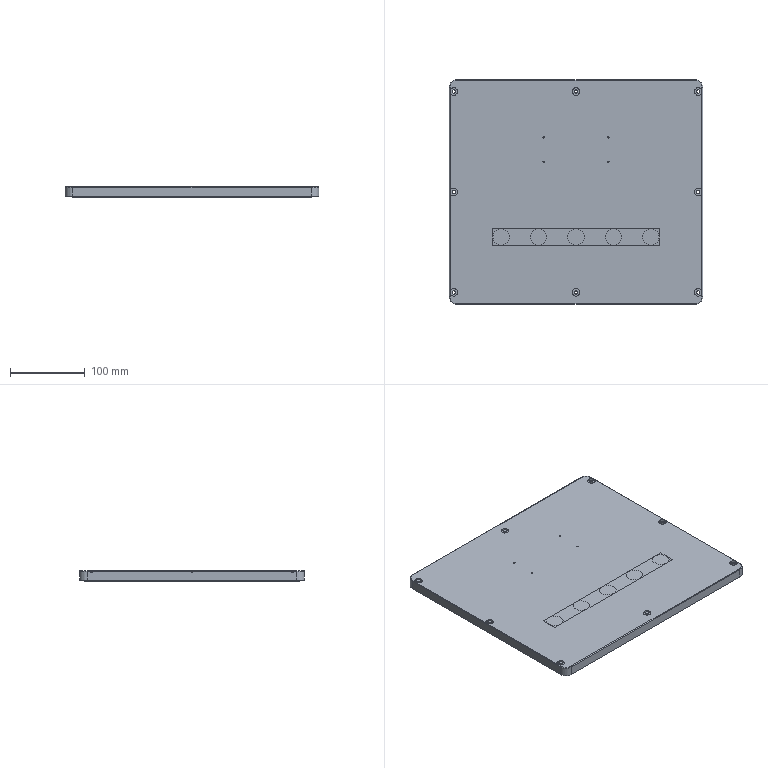NC program | NX | posted with a generic post | part box 338 x 300 x 14.5 mm
Lines 1 to 2601 of 2756, first 2255 of 2575 lines:
N10 G17 G21 G94 G90
(FLOOR_WALL_COPY , TOOL : D63)
N12 T03 M6
N14 G54
N16 G17 G0 G90 X-203.5 Y149.997 S6500 M3
N18 G43 Z30. H3
N20 Z5.662
N22 G94 G1 Z2.662 F1250.
N24 X-200.5
N26 X200.5
N28 Y104.197
N30 X-200.5
N32 Y58.398
N34 X200.5
N36 Y12.599
N38 X-200.5
N40 Y-33.201
N42 X200.5
N44 Y-79.
N46 X-200.5
N48 Y-124.8
N50 X200.5
N52 X203.5
N54 Z5.662
N56 G0 Z30.
N58 X-203.5 Y149.997
N60 Z4.825
N62 G1 Z1.825
N64 X-200.5
N66 X200.5
N68 Y104.197
N70 X-200.5
N72 Y58.398
N74 X200.5
N76 Y12.599
N78 X-200.5
N80 Y-33.201
N82 X200.5
N84 Y-79.
N86 X-200.5
N88 Y-124.8
N90 X200.5
N92 X203.5
N94 Z4.825
N96 G0 Z30.
N98 X-203.5 Y149.997
N100 Z3.987
N102 G1 Z0.987
N104 X-200.5
N106 X200.5
N108 Y104.197
N110 X-200.5
N112 Y58.398
N114 X200.5
N116 Y12.599
N118 X-200.5
N120 Y-33.201
N122 X200.5
N124 Y-79.
N126 X-200.5
N128 Y-124.8
N130 X200.5
N132 X203.5
N134 Z3.987
N136 G0 Z30.
N138 X-203.5 Y149.997
N140 Z3.15
N142 G1 Z0.15
N144 X-200.5
N146 X200.5
N148 Y104.197
N150 X-200.5
N152 Y58.398
N154 X200.5
N156 Y12.599
N158 X-200.5
N160 Y-33.201
N162 X200.5
N164 Y-79.
N166 X-200.5
N168 Y-124.8
N170 X200.5
N172 X203.5
N174 Z3.15
N176 G0 Z30.
(FLOOR_WALL_COPY_1 , TOOL : D63)
N178 X-203.5 Y149.997
N180 Z3.
N182 G1 Z0.
N184 X-200.5
N186 X200.5
N188 Y104.197
N190 X-200.5
N192 Y58.398
N194 X200.5
N196 Y12.599
N198 X-200.5
N200 Y-33.201
N202 X200.5
N204 Y-79.
N206 X-200.5
N208 Y-124.8
N210 X200.5
N212 X203.5
N214 Z3.
N216 G0 Z30.
N218 M5
(CAVITY_MILL_1 , TOOL : D10)
N220 T04 M6
N222 G54
N224 G17 G0 G90 X-3.978 Y-2.05 S9500 M3
N226 G43 Z30. H4
N228 Z1.5
N230 G94 G1 X16.95 Z0.403 F1000.
N232 Y2.05 Z0.188
N234 X0. Z-0.7
N236 X-16.95 F3000.
N238 Y-2.05
N240 X16.95
N242 Y2.05
N244 X0.
N246 Y9.55
N248 X-24.45
N250 Y-9.55
N252 X24.45
N254 Y9.55
N256 X0.
N258 Y17.05
N260 X-31.95
N262 Y-17.05
N264 X31.95
N266 Y17.05
N268 X0.
N270 Y24.55
N272 X-39.45
N274 Y-24.55
N276 X39.45
N278 Y24.55
N280 X0.
N282 Y32.05
N284 X-46.95
N286 Y-32.05
N288 X46.95
N290 Y32.05
N292 X0.
N294 Y39.55
N296 X-54.45
N298 Y-39.55
N300 X54.45
N302 Y39.55
N304 X0.
N306 Y47.05
N308 X-61.95
N310 Y-47.05
N312 X61.95
N314 Y47.05
N316 X0.
N318 Y54.55
N320 X-69.45
N322 Y-54.55
N324 X69.45
N326 Y54.55
N328 X0.
N330 Y62.05
N332 X-76.95
N334 Y-62.05
N336 X76.95
N338 Y62.05
N340 X0.
N342 Y69.55
N344 X-84.45
N346 Y-69.55
N348 X84.45
N350 Y69.55
N352 X0.
N354 Y77.05
N356 X-91.95
N358 Y-77.05
N360 X91.95
N362 Y77.05
N364 X0.
N366 Y84.55
N368 X-99.45
N370 Y-84.55
N372 X99.45
N374 Y84.55
N376 X0.
N378 Y92.05
N380 X-106.95
N382 Y-92.05
N384 X106.95
N386 Y92.05
N388 X0.
N390 Y99.55
N392 X-114.45
N394 Y-99.55
N396 X114.45
N398 Y99.55
N400 X0.
N402 Y107.05
N404 X-121.95
N406 Y-107.05
N408 X121.95
N410 Y107.05
N412 X0.
N414 Y114.55
N416 X-129.45
N418 Y-114.55
N420 X129.45
N422 Y114.55
N424 X0.
N426 Y122.05
N428 X-136.95
N430 Y-122.05
N432 X136.95
N434 Y122.05
N436 X0.
N438 Y129.55
N440 X-144.45
N442 Y-129.55
N444 X144.45
N446 Y129.55
N448 X0.
N450 Y137.05
N452 X-145.05
N454 G3 X-151.95 Y130.15 R6.9
N456 G1 Y-130.15
N458 G3 X-145.05 Y-137.05 R6.9
N460 G1 X145.05
N462 G3 X151.95 Y-130.15 R6.9
N464 G1 Y130.15
N466 G3 X145.05 Y137.05 R6.9
N468 G1 X0.
N470 G3 X-0.866 Y136.55 R1.
N472 G1 Z0.8
N474 G0 Z30.
N476 X-3.978 Y-2.05
N478 Z0.8
N480 G1 X16.95 Z-0.297 F1000.
N482 Y2.05 Z-0.512
N484 X0. Z-1.4
N486 X-16.95 F3000.
N488 Y-2.05
N490 X16.95
N492 Y2.05
N494 X0.
N496 Y9.55
N498 X-24.45
N500 Y-9.55
N502 X24.45
N504 Y9.55
N506 X0.
N508 Y17.05
N510 X-31.95
N512 Y-17.05
N514 X31.95
N516 Y17.05
N518 X0.
N520 Y24.55
N522 X-39.45
N524 Y-24.55
N526 X39.45
N528 Y24.55
N530 X0.
N532 Y32.05
N534 X-46.95
N536 Y-32.05
N538 X46.95
N540 Y32.05
N542 X0.
N544 Y39.55
N546 X-54.45
N548 Y-39.55
N550 X54.45
N552 Y39.55
N554 X0.
N556 Y47.05
N558 X-61.95
N560 Y-47.05
N562 X61.95
N564 Y47.05
N566 X0.
N568 Y54.55
N570 X-69.45
N572 Y-54.55
N574 X69.45
N576 Y54.55
N578 X0.
N580 Y62.05
N582 X-76.95
N584 Y-62.05
N586 X76.95
N588 Y62.05
N590 X0.
N592 Y69.55
N594 X-84.45
N596 Y-69.55
N598 X84.45
N600 Y69.55
N602 X0.
N604 Y77.05
N606 X-91.95
N608 Y-77.05
N610 X91.95
N612 Y77.05
N614 X0.
N616 Y84.55
N618 X-99.45
N620 Y-84.55
N622 X99.45
N624 Y84.55
N626 X0.
N628 Y92.05
N630 X-106.95
N632 Y-92.05
N634 X106.95
N636 Y92.05
N638 X0.
N640 Y99.55
N642 X-114.45
N644 Y-99.55
N646 X114.45
N648 Y99.55
N650 X0.
N652 Y107.05
N654 X-121.95
N656 Y-107.05
N658 X121.95
N660 Y107.05
N662 X0.
N664 Y114.55
N666 X-129.45
N668 Y-114.55
N670 X129.45
N672 Y114.55
N674 X0.
N676 Y122.05
N678 X-136.95
N680 Y-122.05
N682 X136.95
N684 Y122.05
N686 X0.
N688 Y129.55
N690 X-144.45
N692 Y-129.55
N694 X144.45
N696 Y129.55
N698 X0.
N700 Y137.05
N702 X-145.05
N704 G3 X-151.95 Y130.15 R6.9
N706 G1 Y-130.15
N708 G3 X-145.05 Y-137.05 R6.9
N710 G1 X145.05
N712 G3 X151.95 Y-130.15 R6.9
N714 G1 Y130.15
N716 G3 X145.05 Y137.05 R6.9
N718 G1 X0.
N720 G3 X-0.866 Y136.55 R1.
N722 G1 Z0.1
N724 G0 Z30.
N726 X-10.103 Y-1.9
N728 Z0.1
N730 G1 X16.9 Z-1.315 F1000.
N732 Y1.9 Z-1.514
N734 X0. Z-2.4
N736 X-16.9 F3000.
N738 Y-1.9
N740 X16.9
N742 Y1.9
N744 X0.
N746 Y6.4
N748 X-21.4
N750 Y-6.4
N752 X21.4
N754 Y6.4
N756 X0.
N758 Y13.9
N760 X-28.9
N762 Y-13.9
N764 X28.9
N766 Y13.9
N768 X0.
N770 Y21.4
N772 X-36.4
N774 Y-21.4
N776 X36.4
N778 Y21.4
N780 X0.
N782 Y28.9
N784 X-43.9
N786 Y-28.9
N788 X43.9
N790 Y28.9
N792 X0.
N794 Y36.4
N796 X-51.4
N798 Y-36.4
N800 X51.4
N802 Y36.4
N804 X0.
N806 Y43.9
N808 X-58.9
N810 Y-43.9
N812 X58.9
N814 Y43.9
N816 X0.
N818 Y51.4
N820 X-66.4
N822 Y-51.4
N824 X66.4
N826 Y51.4
N828 X0.
N830 Y58.9
N832 X-73.9
N834 Y-58.9
N836 X73.9
N838 Y58.9
N840 X0.
N842 Y66.4
N844 X-81.4
N846 Y-66.4
N848 X81.4
N850 Y66.4
N852 X0.
N854 Y73.9
N856 X-88.9
N858 Y-73.9
N860 X88.9
N862 Y73.9
N864 X0.
N866 Y81.4
N868 X-96.4
N870 Y-81.4
N872 X96.4
N874 Y81.4
N876 X0.
N878 Y88.9
N880 X-103.9
N882 Y-88.9
N884 X103.9
N886 Y88.9
N888 X0.
N890 Y96.4
N892 X-111.4
N894 Y-96.4
N896 X111.4
N898 Y96.4
N900 X0.
N902 Y103.9
N904 X-118.9
N906 Y-103.9
N908 X118.9
N910 Y103.9
N912 X0.
N914 Y111.4
N916 X-126.4
N918 Y-111.4
N920 X126.4
N922 Y111.4
N924 X0.
N926 Y118.9
N928 X-133.9
N930 Y-118.9
N932 X133.9
N934 Y118.9
N936 X0.
N938 Y126.4
N940 X-141.4
N942 Y-126.4
N944 X141.4
N946 Y126.4
N948 X0.
N950 Y133.9
N952 X-144.
N954 G3 X-148.9 Y129. R4.9
N956 G1 Y-129.
N958 G3 X-144. Y-133.9 R4.9
N960 G1 X144.
N962 G3 X148.9 Y-129. R4.9
N964 G1 Y129.
N966 G3 X144. Y133.9 R4.9
N968 G1 X0.
N970 G3 X-0.866 Y133.4 R1.
N972 G1 Z-0.9
N974 G0 X-10.103 Y-1.9
N976 G1 X16.9 Z-2.315 F1000.
N978 Y1.9 Z-2.514
N980 X0. Z-3.4
N982 X-16.9 F3000.
N984 Y-1.9
N986 X16.9
N988 Y1.9
N990 X0.
N992 Y6.4
N994 X-21.4
N996 Y-6.4
N998 X21.4
N1000 Y6.4
N1002 X0.
N1004 Y13.9
N1006 X-28.9
N1008 Y-13.9
N1010 X28.9
N1012 Y13.9
N1014 X0.
N1016 Y21.4
N1018 X-36.4
N1020 Y-21.4
N1022 X36.4
N1024 Y21.4
N1026 X0.
N1028 Y28.9
N1030 X-43.9
N1032 Y-28.9
N1034 X43.9
N1036 Y28.9
N1038 X0.
N1040 Y36.4
N1042 X-51.4
N1044 Y-36.4
N1046 X51.4
N1048 Y36.4
N1050 X0.
N1052 Y43.9
N1054 X-58.9
N1056 Y-43.9
N1058 X58.9
N1060 Y43.9
N1062 X0.
N1064 Y51.4
N1066 X-66.4
N1068 Y-51.4
N1070 X66.4
N1072 Y51.4
N1074 X0.
N1076 Y58.9
N1078 X-73.9
N1080 Y-58.9
N1082 X73.9
N1084 Y58.9
N1086 X0.
N1088 Y66.4
N1090 X-81.4
N1092 Y-66.4
N1094 X81.4
N1096 Y66.4
N1098 X0.
N1100 Y73.9
N1102 X-88.9
N1104 Y-73.9
N1106 X88.9
N1108 Y73.9
N1110 X0.
N1112 Y81.4
N1114 X-96.4
N1116 Y-81.4
N1118 X96.4
N1120 Y81.4
N1122 X0.
N1124 Y88.9
N1126 X-103.9
N1128 Y-88.9
N1130 X103.9
N1132 Y88.9
N1134 X0.
N1136 Y96.4
N1138 X-111.4
N1140 Y-96.4
N1142 X111.4
N1144 Y96.4
N1146 X0.
N1148 Y103.9
N1150 X-118.9
N1152 Y-103.9
N1154 X118.9
N1156 Y103.9
N1158 X0.
N1160 Y111.4
N1162 X-126.4
N1164 Y-111.4
N1166 X126.4
N1168 Y111.4
N1170 X0.
N1172 Y118.9
N1174 X-133.9
N1176 Y-118.9
N1178 X133.9
N1180 Y118.9
N1182 X0.
N1184 Y126.4
N1186 X-141.4
N1188 Y-126.4
N1190 X141.4
N1192 Y126.4
N1194 X0.
N1196 Y133.9
N1198 X-144.
N1200 G3 X-148.9 Y129. R4.9
N1202 G1 Y-129.
N1204 G3 X-144. Y-133.9 R4.9
N1206 G1 X144.
N1208 G3 X148.9 Y-129. R4.9
N1210 G1 Y129.
N1212 G3 X144. Y133.9 R4.9
N1214 G1 X0.
N1216 G3 X-0.866 Y133.4 R1.
N1218 G1 Z-1.9
N1220 G0 X-10.103 Y-1.9
N1222 G1 X16.9 Z-3.315 F1000.
N1224 Y1.9 Z-3.514
N1226 X0. Z-4.4
N1228 X-16.9 F3000.
N1230 Y-1.9
N1232 X16.9
N1234 Y1.9
N1236 X0.
N1238 Y6.4
N1240 X-21.4
N1242 Y-6.4
N1244 X21.4
N1246 Y6.4
N1248 X0.
N1250 Y13.9
N1252 X-28.9
N1254 Y-13.9
N1256 X28.9
N1258 Y13.9
N1260 X0.
N1262 Y21.4
N1264 X-36.4
N1266 Y-21.4
N1268 X36.4
N1270 Y21.4
N1272 X0.
N1274 Y28.9
N1276 X-43.9
N1278 Y-28.9
N1280 X43.9
N1282 Y28.9
N1284 X0.
N1286 Y36.4
N1288 X-51.4
N1290 Y-36.4
N1292 X51.4
N1294 Y36.4
N1296 X0.
N1298 Y43.9
N1300 X-58.9
N1302 Y-43.9
N1304 X58.9
N1306 Y43.9
N1308 X0.
N1310 Y51.4
N1312 X-66.4
N1314 Y-51.4
N1316 X66.4
N1318 Y51.4
N1320 X0.
N1322 Y58.9
N1324 X-73.9
N1326 Y-58.9
N1328 X73.9
N1330 Y58.9
N1332 X0.
N1334 Y66.4
N1336 X-81.4
N1338 Y-66.4
N1340 X81.4
N1342 Y66.4
N1344 X0.
N1346 Y73.9
N1348 X-88.9
N1350 Y-73.9
N1352 X88.9
N1354 Y73.9
N1356 X0.
N1358 Y81.4
N1360 X-96.4
N1362 Y-81.4
N1364 X96.4
N1366 Y81.4
N1368 X0.
N1370 Y88.9
N1372 X-103.9
N1374 Y-88.9
N1376 X103.9
N1378 Y88.9
N1380 X0.
N1382 Y96.4
N1384 X-111.4
N1386 Y-96.4
N1388 X111.4
N1390 Y96.4
N1392 X0.
N1394 Y103.9
N1396 X-118.9
N1398 Y-103.9
N1400 X118.9
N1402 Y103.9
N1404 X0.
N1406 Y111.4
N1408 X-126.4
N1410 Y-111.4
N1412 X126.4
N1414 Y111.4
N1416 X0.
N1418 Y118.9
N1420 X-133.9
N1422 Y-118.9
N1424 X133.9
N1426 Y118.9
N1428 X0.
N1430 Y126.4
N1432 X-141.4
N1434 Y-126.4
N1436 X141.4
N1438 Y126.4
N1440 X0.
N1442 Y133.9
N1444 X-144.
N1446 G3 X-148.9 Y129. R4.9
N1448 G1 Y-129.
N1450 G3 X-144. Y-133.9 R4.9
N1452 G1 X144.
N1454 G3 X148.9 Y-129. R4.9
N1456 G1 Y129.
N1458 G3 X144. Y133.9 R4.9
N1460 G1 X0.
N1462 G3 X-0.866 Y133.4 R1.
N1464 G1 Z-2.9
N1466 G0 X-10.103 Y-1.9
N1468 G1 X16.9 Z-4.315 F1000.
N1470 Y1.9 Z-4.514
N1472 X0. Z-5.4
N1474 X-16.9 F3000.
N1476 Y-1.9
N1478 X16.9
N1480 Y1.9
N1482 X0.
N1484 Y6.4
N1486 X-21.4
N1488 Y-6.4
N1490 X21.4
N1492 Y6.4
N1494 X0.
N1496 Y13.9
N1498 X-28.9
N1500 Y-13.9
N1502 X28.9
N1504 Y13.9
N1506 X0.
N1508 Y21.4
N1510 X-36.4
N1512 Y-21.4
N1514 X36.4
N1516 Y21.4
N1518 X0.
N1520 Y28.9
N1522 X-43.9
N1524 Y-28.9
N1526 X43.9
N1528 Y28.9
N1530 X0.
N1532 Y36.4
N1534 X-51.4
N1536 Y-36.4
N1538 X51.4
N1540 Y36.4
N1542 X0.
N1544 Y43.9
N1546 X-58.9
N1548 Y-43.9
N1550 X58.9
N1552 Y43.9
N1554 X0.
N1556 Y51.4
N1558 X-66.4
N1560 Y-51.4
N1562 X66.4
N1564 Y51.4
N1566 X0.
N1568 Y58.9
N1570 X-73.9
N1572 Y-58.9
N1574 X73.9
N1576 Y58.9
N1578 X0.
N1580 Y66.4
N1582 X-81.4
N1584 Y-66.4
N1586 X81.4
N1588 Y66.4
N1590 X0.
N1592 Y73.9
N1594 X-88.9
N1596 Y-73.9
N1598 X88.9
N1600 Y73.9
N1602 X0.
N1604 Y81.4
N1606 X-96.4
N1608 Y-81.4
N1610 X96.4
N1612 Y81.4
N1614 X0.
N1616 Y88.9
N1618 X-103.9
N1620 Y-88.9
N1622 X103.9
N1624 Y88.9
N1626 X0.
N1628 Y96.4
N1630 X-111.4
N1632 Y-96.4
N1634 X111.4
N1636 Y96.4
N1638 X0.
N1640 Y103.9
N1642 X-118.9
N1644 Y-103.9
N1646 X118.9
N1648 Y103.9
N1650 X0.
N1652 Y111.4
N1654 X-126.4
N1656 Y-111.4
N1658 X126.4
N1660 Y111.4
N1662 X0.
N1664 Y118.9
N1666 X-133.9
N1668 Y-118.9
N1670 X133.9
N1672 Y118.9
N1674 X0.
N1676 Y126.4
N1678 X-141.4
N1680 Y-126.4
N1682 X141.4
N1684 Y126.4
N1686 X0.
N1688 Y133.9
N1690 X-144.
N1692 G3 X-148.9 Y129. R4.9
N1694 G1 Y-129.
N1696 G3 X-144. Y-133.9 R4.9
N1698 G1 X144.
N1700 G3 X148.9 Y-129. R4.9
N1702 G1 Y129.
N1704 G3 X144. Y133.9 R4.9
N1706 G1 X0.
N1708 G3 X-0.866 Y133.4 R1.
N1710 G1 Z-3.9
N1712 G0 X17.397 Y6.6
N1714 G1 X28.9 Z-4.503 F1000.
N1716 Y13.9 Z-4.885
N1718 X0. Z-6.4
N1720 X-28.9 F3000.
N1722 Y6.6
N1724 X28.9
N1726 Y13.9
N1728 X0.
N1730 Y21.4
N1732 X-36.4
N1734 Y-0.9
N1736 X36.4
N1738 Y21.4
N1740 X0.
N1742 Y28.9
N1744 X-43.9
N1746 Y-8.4
N1748 X43.9
N1750 Y28.9
N1752 X0.
N1754 Y36.4
N1756 X-51.4
N1758 Y-15.9
N1760 X51.4
N1762 Y36.4
N1764 X0.
N1766 Y43.9
N1768 X-58.9
N1770 Y-23.4
N1772 X58.9
N1774 Y43.9
N1776 X0.
N1778 Y51.4
N1780 X-66.4
N1782 Y-30.9
N1784 X66.4
N1786 Y51.4
N1788 X0.
N1790 Y58.9
N1792 X-73.9
N1794 Y-38.4
N1796 X73.9
N1798 Y58.9
N1800 X0.
N1802 Y66.4
N1804 X-81.4
N1806 Y-45.9
N1808 X81.4
N1810 Y66.4
N1812 X0.
N1814 Y73.9
N1816 X-88.9
N1818 Y-53.4
N1820 X88.9
N1822 Y73.9
N1824 X0.
N1826 Y81.4
N1828 X-96.4
N1830 Y-60.9
N1832 X96.4
N1834 Y81.4
N1836 X0.
N1838 Y88.9
N1840 X-103.9
N1842 Y-68.4
N1844 X103.9
N1846 Y88.9
N1848 X0.
N1850 Y96.4
N1852 X-111.4
N1854 Y-77.004
N1856 G2 X-105. Y-75.9 R19.1
N1858 G1 X105.
N1860 G2 X111.4 Y-77.004 R19.1
N1862 G1 Y96.4
N1864 X0.
N1866 Y103.9
N1868 X-118.9
N1870 Y-103.9
N1872 X-112.44
N1874 X-107.761 Y-106.337
N1876 X-112.44 Y-103.9
N1878 G2 X-105. Y-83.4 R11.6
N1880 G1 X105.
N1882 G2 X112.44 Y-103.9 R11.6
N1884 G1 X107.761 Y-106.337
N1886 X112.44 Y-103.9
N1888 X111.478 Y-102.749
N1890 G2 X105. Y-105.1 R10.1
N1892 G1 X-105.
N1894 G2 X-115.1 Y-95. R10.1
N1896 X-105. Y-84.9 R10.1
N1898 G1 X105.
N1900 G2 X111.478 Y-102.749 R10.1
N1902 G1 X112.44 Y-103.9
N1904 X118.9
N1906 Y103.9
N1908 X0.
N1910 Y111.4
N1912 X-126.4
N1914 Y-111.4
N1916 X126.4
N1918 Y111.4
N1920 X0.
N1922 Y118.9
N1924 X-133.9
N1926 Y-118.9
N1928 X133.9
N1930 Y118.9
N1932 X0.
N1934 Y126.4
N1936 X-141.4
N1938 Y-126.4
N1940 X141.4
N1942 Y126.4
N1944 X0.
N1946 Y133.9
N1948 X-144.
N1950 G3 X-148.9 Y129. R4.9
N1952 G1 Y-129.
N1954 G3 X-144. Y-133.9 R4.9
N1956 G1 X144.
N1958 G3 X148.9 Y-129. R4.9
N1960 G1 Y129.
N1962 G3 X144. Y133.9 R4.9
N1964 G1 X0.
N1966 G3 X-0.866 Y133.4 R1.
N1968 G1 Z-4.9
N1970 G0 X17.397 Y6.6
N1972 G1 X28.9 Z-5.503 F1000.
N1974 Y13.9 Z-5.885
N1976 X0. Z-7.4
N1978 X-28.9 F3000.
N1980 Y6.6
N1982 X28.9
N1984 Y13.9
N1986 X0.
N1988 Y21.4
N1990 X-36.4
N1992 Y-0.9
N1994 X36.4
N1996 Y21.4
N1998 X0.
N2000 Y28.9
N2002 X-43.9
N2004 Y-8.4
N2006 X43.9
N2008 Y28.9
N2010 X0.
N2012 Y36.4
N2014 X-51.4
N2016 Y-15.9
N2018 X51.4
N2020 Y36.4
N2022 X0.
N2024 Y43.9
N2026 X-58.9
N2028 Y-23.4
N2030 X58.9
N2032 Y43.9
N2034 X0.
N2036 Y51.4
N2038 X-66.4
N2040 Y-30.9
N2042 X66.4
N2044 Y51.4
N2046 X0.
N2048 Y58.9
N2050 X-73.9
N2052 Y-38.4
N2054 X73.9
N2056 Y58.9
N2058 X0.
N2060 Y66.4
N2062 X-81.4
N2064 Y-45.9
N2066 X81.4
N2068 Y66.4
N2070 X0.
N2072 Y73.9
N2074 X-88.9
N2076 Y-53.4
N2078 X88.9
N2080 Y73.9
N2082 X0.
N2084 Y81.4
N2086 X-96.4
N2088 Y-60.9
N2090 X96.4
N2092 Y81.4
N2094 X0.
N2096 Y88.9
N2098 X-103.9
N2100 Y-68.4
N2102 X103.9
N2104 Y88.9
N2106 X0.
N2108 Y96.4
N2110 X-111.4
N2112 Y-77.004
N2114 G2 X-105. Y-75.9 R19.1
N2116 G1 X105.
N2118 G2 X111.4 Y-77.004 R19.1
N2120 G1 Y96.4
N2122 X0.
N2124 Y103.9
N2126 X-118.9
N2128 Y-103.9
N2130 X-112.44
N2132 X-107.761 Y-106.337
N2134 X-112.44 Y-103.9
N2136 G2 X-105. Y-83.4 R11.6
N2138 G1 X105.
N2140 G2 X112.44 Y-103.9 R11.6
N2142 G1 X107.761 Y-106.337
N2144 X112.44 Y-103.9
N2146 X111.478 Y-102.749
N2148 G2 X105. Y-105.1 R10.1
N2150 G1 X-105.
N2152 G2 X-115.1 Y-95. R10.1
N2154 X-105. Y-84.9 R10.1
N2156 G1 X105.
N2158 G2 X111.478 Y-102.749 R10.1
N2160 G1 X112.44 Y-103.9
N2162 X118.9
N2164 Y103.9
N2166 X0.
N2168 Y111.4
N2170 X-126.4
N2172 Y-111.4
N2174 X126.4
N2176 Y111.4
N2178 X0.
N2180 Y118.9
N2182 X-133.9
N2184 Y-118.9
N2186 X133.9
N2188 Y118.9
N2190 X0.
N2192 Y126.4
N2194 X-141.4
N2196 Y-126.4
N2198 X141.4
N2200 Y126.4
N2202 X0.
N2204 Y133.9
N2206 X-144.
N2208 G3 X-148.9 Y129. R4.9
N2210 G1 Y-129.
N2212 G3 X-144. Y-133.9 R4.9
N2214 G1 X144.
N2216 G3 X148.9 Y-129. R4.9
N2218 G1 Y129.
N2220 G3 X144. Y133.9 R4.9
N2222 G1 X0.
N2224 G3 X-0.866 Y133.4 R1.
N2226 G1 Z-5.9
N2228 G0 X17.397 Y6.6
N2230 G1 X28.9 Z-6.503 F1000.
N2232 Y13.9 Z-6.885
N2234 X0. Z-8.4
N2236 X-28.9 F3000.
N2238 Y6.6
N2240 X28.9
N2242 Y13.9
N2244 X0.
N2246 Y21.4
N2248 X-36.4
N2250 Y-0.9
N2252 X36.4
N2254 Y21.4
N2256 X0.
N2258 Y28.9
N2260 X-43.9
N2262 Y-8.4
N2264 X43.9
N2266 Y28.9
N2268 X0.
N2270 Y36.4
N2272 X-51.4
N2274 Y-15.9
N2276 X51.4
N2278 Y36.4
N2280 X0.
N2282 Y43.9
N2284 X-58.9
N2286 Y-23.4
N2288 X58.9
N2290 Y43.9
N2292 X0.
N2294 Y51.4
N2296 X-66.4
N2298 Y-30.9
N2300 X66.4
N2302 Y51.4
N2304 X0.
N2306 Y58.9
N2308 X-73.9
N2310 Y-38.4
N2312 X73.9
N2314 Y58.9
N2316 X0.
N2318 Y66.4
N2320 X-81.4
N2322 Y-45.9
N2324 X81.4
N2326 Y66.4
N2328 X0.
N2330 Y73.9
N2332 X-88.9
N2334 Y-53.4
N2336 X88.9
N2338 Y73.9
N2340 X0.
N2342 Y81.4
N2344 X-96.4
N2346 Y-60.9
N2348 X96.4
N2350 Y81.4
N2352 X0.
N2354 Y88.9
N2356 X-103.9
N2358 Y-68.4
N2360 X103.9
N2362 Y88.9
N2364 X0.
N2366 Y96.4
N2368 X-111.4
N2370 Y-77.004
N2372 G2 X-105. Y-75.9 R19.1
N2374 G1 X105.
N2376 G2 X111.4 Y-77.004 R19.1
N2378 G1 Y96.4
N2380 X0.
N2382 Y103.9
N2384 X-118.9
N2386 Y-103.9
N2388 X-112.44
N2390 X-107.761 Y-106.337
N2392 X-112.44 Y-103.9
N2394 G2 X-105. Y-83.4 R11.6
N2396 G1 X105.
N2398 G2 X112.44 Y-103.9 R11.6
N2400 G1 X107.761 Y-106.337
N2402 X112.44 Y-103.9
N2404 X111.478 Y-102.749
N2406 G2 X105. Y-105.1 R10.1
N2408 G1 X-105.
N2410 G2 X-115.1 Y-95. R10.1
N2412 X-105. Y-84.9 R10.1
N2414 G1 X105.
N2416 G2 X111.478 Y-102.749 R10.1
N2418 G1 X112.44 Y-103.9
N2420 X118.9
N2422 Y103.9
N2424 X0.
N2426 Y111.4
N2428 X-126.4
N2430 Y-111.4
N2432 X126.4
N2434 Y111.4
N2436 X0.
N2438 Y118.9
N2440 X-133.9
N2442 Y-118.9
N2444 X133.9
N2446 Y118.9
N2448 X0.
N2450 Y126.4
N2452 X-141.4
N2454 Y-126.4
N2456 X141.4
N2458 Y126.4
N2460 X0.
N2462 Y133.9
N2464 X-144.
N2466 G3 X-148.9 Y129. R4.9
N2468 G1 Y-129.
N2470 G3 X-144. Y-133.9 R4.9
N2472 G1 X144.
N2474 G3 X148.9 Y-129. R4.9
N2476 G1 Y129.
N2478 G3 X144. Y133.9 R4.9
N2480 G1 X0.
N2482 G3 X-0.866 Y133.4 R1.
N2484 G1 Z-6.9
N2486 G0 X17.397 Y6.6
N2488 G1 X28.9 Z-7.503 F1000.
N2490 Y13.9 Z-7.885
N2492 X0. Z-9.4
N2494 X-28.9 F3000.
N2496 Y6.6
N2498 X28.9
N2500 Y13.9
N2502 X0.
N2504 Y21.4
N2506 X-36.4
N2508 Y-0.9
N2510 X36.4
N2512 Y21.4
N2514 X0.
N2516 Y28.9
N2518 X-43.9
N2520 Y-8.4
N2522 X43.9
N2524 Y28.9
N2526 X0.
N2528 Y36.4
N2530 X-51.4
N2532 Y-15.9
N2534 X51.4
N2536 Y36.4
N2538 X0.
N2540 Y43.9
N2542 X-58.9
N2544 Y-23.4
N2546 X58.9
N2548 Y43.9
N2550 X0.
N2552 Y51.4
N2554 X-66.4
N2556 Y-30.9
N2558 X66.4
N2560 Y51.4
N2562 X0.
N2564 Y58.9
N2566 X-73.9
N2568 Y-38.4
N2570 X73.9
N2572 Y58.9
N2574 X0.
N2576 Y66.4
N2578 X-81.4
N2580 Y-45.9
N2582 X81.4
N2584 Y66.4
N2586 X0.
N2588 Y73.9
N2590 X-88.9
N2592 Y-53.4
N2594 X88.9
N2596 Y73.9
N2598 X0.
N2600 Y81.4
N2602 X-96.4
N2604 Y-60.9
N2606 X96.4
N2608 Y81.4
N2610 X0.
N2612 Y88.9
N2614 X-103.9
N2616 Y-68.4
N2618 X103.9
N2620 Y88.9
N2622 X0.
N2624 Y96.4
N2626 X-111.4
N2628 Y-77.004
N2630 G2 X-105. Y-75.9 R19.1
N2632 G1 X105.
N2634 G2 X111.4 Y-77.004 R19.1
N2636 G1 Y96.4
N2638 X0.
N2640 Y103.9
N2642 X-118.9
N2644 Y-103.9
N2646 X-112.44
N2648 X-107.761 Y-106.337
N2650 X-112.44 Y-103.9
N2652 G2 X-105. Y-83.4 R11.6
N2654 G1 X105.
N2656 G2 X112.44 Y-103.9 R11.6
N2658 G1 X107.761 Y-106.337
N2660 X112.44 Y-103.9
N2662 X111.478 Y-102.749
N2664 G2 X105. Y-105.1 R10.1
N2666 G1 X-105.
N2668 G2 X-115.1 Y-95. R10.1
N2670 X-105. Y-84.9 R10.1
N2672 G1 X105.
N2674 G2 X111.478 Y-102.749 R10.1
N2676 G1 X112.44 Y-103.9
N2678 X118.9
N2680 Y103.9
N2682 X0.
N2684 Y111.4
N2686 X-126.4
N2688 Y-111.4
N2690 X126.4
N2692 Y111.4
N2694 X0.
N2696 Y118.9
N2698 X-133.9
N2700 Y-118.9
N2702 X133.9
N2704 Y118.9
N2706 X0.
N2708 Y126.4
N2710 X-141.4
N2712 Y-126.4
N2714 X141.4
N2716 Y126.4
N2718 X0.
N2720 Y133.9
N2722 X-144.
N2724 G3 X-148.9 Y129. R4.9
N2726 G1 Y-129.
N2728 G3 X-144. Y-133.9 R4.9
N2730 G1 X144.
N2732 G3 X148.9 Y-129. R4.9
N2734 G1 Y129.
N2736 G3 X144. Y133.9 R4.9
N2738 G1 X0.
N2740 G3 X-0.866 Y133.4 R1.
N2742 G1 Z-7.9
N2744 G0 Z30.
(FLOOR_WALL_1 , TOOL : D10)
N2746 X177. Y5.196
N2748 Z0.8
N2750 G1 Z-0.7 F1000.
N2752 X169.5 Y0.866
N2754 G3 X169. Y0. R1.
N2756 G1 Y-140. F2500.
N2758 G2 X159. Y-150. R10.
N2760 G1 X148.794
N2762 G3 X165.25 Y-130.15 R20.2
N2764 G1 Y130.15
N2766 G3 X148.794 Y150. R20.2
N2768 G1 X159.
N2770 G2 X169. Y140. R10.
N2772 G1 Y0.
N2774 G3 X169.5 Y-0.866 R1.
N2776 G1 X177. Y-5.196
N2778 Z0.8
N2780 G0 Z30.
N2782 X-177.
N2784 Z0.8
N2786 G1 Z-0.7 F1000.
N2788 X-169.5 Y-0.866
N2790 G3 X-169. Y0. R1.
N2792 G1 Y140. F2500.
N2794 G2 X-159. Y150. R10.
N2796 G1 X-148.794
N2798 G3 X-165.25 Y130.15 R20.2
N2800 G1 Y-130.15
N2802 G3 X-148.794 Y-150. R20.2
N2804 G1 X-148.535 Y-148.624
N2806 G2 X-163.85 Y-130.15 R18.8
N2808 G1 Y130.15
N2810 G2 X-145.05 Y148.95 R18.8
N2812 G1 X145.05
N2814 G2 X163.85 Y130.15 R18.8
N2816 G1 Y-130.15
N2818 G2 X145.05 Y-148.95 R18.8
N2820 G1 X-145.05
N2822 G2 X-148.535 Y-148.624 R18.8
N2824 G1 X-148.794 Y-150.
N2826 X-159.
N2828 G2 X-169. Y-140. R10.
N2830 G1 Y0.
N2832 G3 X-169.5 Y0.866 R1.
N2834 G1 X-177. Y5.196
N2836 Z0.8
N2838 G0 Y-5.196 Z0.1
N2840 G1 Z-1.4 F1000.
N2842 X-169.5 Y-0.866
N2844 G3 X-169. Y0. R1.
N2846 G1 Y140. F2500.
N2848 G2 X-159. Y150. R10.
N2850 G1 X-148.794
N2852 G3 X-165.25 Y130.15 R20.2
N2854 G1 Y-130.15
N2856 G3 X-148.794 Y-150. R20.2
N2858 G1 X-159.
N2860 G2 X-169. Y-140. R10.
N2862 G1 Y0.
N2864 G3 X-169.5 Y0.866 R1.
N2866 G1 X-177. Y5.196
N2868 Z0.1
N2870 G0 Z30.
N2872 X177.
N2874 Z0.1
N2876 G1 Z-1.4 F1000.
N2878 X169.5 Y0.866
N2880 G3 X169. Y0. R1.
N2882 G1 Y-140. F2500.
N2884 G2 X159. Y-150. R10.
N2886 G1 X148.794
N2888 G3 X165.25 Y-130.15 R20.2
N2890 G1 Y130.15
N2892 G3 X148.794 Y150. R20.2
N2894 G1 X148.535 Y148.624
N2896 G2 X163.85 Y130.15 R18.8
N2898 G1 Y-130.15
N2900 G2 X145.05 Y-148.95 R18.8
N2902 G1 X-145.05
N2904 G2 X-163.85 Y-130.15 R18.8
N2906 G1 Y130.15
N2908 G2 X-145.05 Y148.95 R18.8
N2910 G1 X145.05
N2912 G2 X148.535 Y148.624 R18.8
N2914 G1 X148.794 Y150.
N2916 X159.
N2918 G2 X169. Y140. R10.
N2920 G1 Y0.
N2922 G3 X169.5 Y-0.866 R1.
N2924 G1 X177. Y-5.196
N2926 Z0.1
N2928 G0 Z30.
N2930 M5
(DRILLING_COPY_1_1 , TOOL : D6A45)
N2932 T01 M6
N2934 G54
N2936 G17 G0 G90 X75. Y-95. S5000 M3
N2938 G43 Z30. H1
N2940 G94 G81 G98 Z-6.1 F250. R-2.5
N2942 X25.
N2944 X-25.
N2946 X-75.
N2948 G80
N2950 G0 X-75. Y-95. Z30.
N2952 M5
(DRILLING_COPY_COPY_1 , TOOL : 2.5ZT)
N2954 T22 M6
N2956 G54
N2958 G17 G0 G90 X75. Y-95. S1447 M3
N2960 G43 Z30. H22
N2962 G94 G83 G98 Z-12.251 F100. Q2. R-2.5
N2964 X25.
N2966 X-25.
N2968 X-75.
N2970 G80
N2972 G0 X-75. Y-95. Z30.
N2974 M5
(FLOOR_WALL_1_COPY_1 , TOOL : D10JING)
N2976 T14 M6
N2978 G54
N2980 G17 G0 G90 X-114.819 Y-89.014 S9500 M3
N2982 G43 Z30. H14
N2984 Z-4.
N2986 G94 G1 Z-5.5 F1000.
N2988 X-114.533 Y-89.511
N2990 G3 X-113.666 Y-90.011 R1.
N2992 G1 X113.661 Y-90.001 F1200.
N2994 G2 X114.95 Y-96. R10.
N2996 G1 X-114.949 Y-96.01
N2998 G2 X-115.815 Y-95.51 R1.
N3000 G1 X-116.482 Y-94.355
N3002 Z-4.
N3004 G0 Z30.
N3006 X-171.322 Y150.974
N3008 Z0.
N3010 G1 Z-1.5 F1000.
N3012 X-171.047 Y150.499
N3014 G3 X-170.181 Y149.999 R1.
N3016 G1 X170.181 F1200.
N3018 G2 X173.435 Y144.079 R15.
N3020 G1 X158.264
N3022 G2 X162.5 Y138.159 R19.2
N3024 G1 X174.
N3026 Y132.239
N3028 X164.136
N3030 G2 X164.25 Y130.15 R19.2
N3032 G1 Y126.319
N3034 X174.
N3036 Y120.399
N3038 X164.25
N3040 Y114.479
N3042 X174.
N3044 Y108.559
N3046 X164.25
N3048 Y102.639
N3050 X174.
N3052 Y96.719
N3054 X164.25
N3056 Y90.799
N3058 X174.
N3060 Y84.879
N3062 X164.25
N3064 Y78.959
N3066 X174.
N3068 Y73.039
N3070 X164.25
N3072 Y67.119
N3074 X174.
N3076 Y61.199
N3078 X164.25
N3080 Y55.279
N3082 X174.
N3084 Y49.359
N3086 X164.25
N3088 Y43.439
N3090 X174.
N3092 Y37.519
N3094 X164.25
N3096 Y31.599
N3098 X174.
N3100 Y25.679
N3102 X164.25
N3104 Y19.759
N3106 X174.
N3108 Y13.839
N3110 X164.25
N3112 Y7.919
N3114 X174.
N3116 Y2.
N3118 X164.25
N3120 Y-3.92
N3122 X174.
N3124 Y-9.84
N3126 X164.25
N3128 Y-15.76
N3130 X174.
N3132 Y-21.68
N3134 X164.25
N3136 Y-27.6
N3138 X174.
N3140 Y-33.52
N3142 X164.25
N3144 Y-39.44
N3146 X174.
N3148 Y-45.36
N3150 X164.25
N3152 Y-51.28
N3154 X174.
N3156 Y-57.2
N3158 X164.25
N3160 Y-63.12
N3162 X174.
N3164 Y-69.04
N3166 X164.25
N3168 Y-74.96
N3170 X174.
N3172 Y-80.88
N3174 X164.25
N3176 Y-86.8
N3178 X174.
N3180 Y-92.72
N3182 X164.25
N3184 Y-98.64
N3186 X174.
N3188 Y-104.56
N3190 X164.25
N3192 Y-110.48
N3194 X174.
N3196 Y-116.4
N3198 X164.25
N3200 Y-122.32
N3202 X174.
N3204 Y-128.24
N3206 X164.25
N3208 Y-130.15
N3210 G2 X163.827 Y-134.16 R19.2
N3212 G1 X174.
N3214 Y-140.
N3216 Y-140.08
N3218 X161.483
N3220 G2 X155.886 Y-146. R19.2
N3222 G1 X172.748
N3224 G3 X173.614 Y-145.5 R1.
N3226 G1 X174.443 Y-145.812
N3228 Z0.
N3230 G0 Z1.6
N3232 G1 X158.264 Y144.079 F8000.
N3234 G0 Z0.
N3236 G1 Z-1.5 F1000.
N3238 G3 X145.05 Y149.35 R19.2
N3240 G1 X-145.05
N3242 G3 X-158.264 Y144.079 R19.2
N3244 G1 X-173.435 F1200.
N3246 G3 X-174. Y140. R15.
N3248 G1 Y138.159
N3250 X-162.5
N3252 G3 X-164.136 Y132.239 R19.2
N3254 G1 X-174.
N3256 Y126.319
N3258 X-164.25
N3260 Y120.399
N3262 X-174.
N3264 Y114.479
N3266 X-164.25
N3268 Y108.559
N3270 X-174.
N3272 Y102.639
N3274 X-164.25
N3276 Y96.719
N3278 X-174.
N3280 Y90.799
N3282 X-164.25
N3284 Y84.879
N3286 X-174.
N3288 Y78.959
N3290 X-164.25
N3292 Y73.039
N3294 X-174.
N3296 Y67.119
N3298 X-164.25
N3300 Y61.199
N3302 X-174.
N3304 Y55.279
N3306 X-164.25
N3308 Y49.359
N3310 X-174.
N3312 Y43.439
N3314 X-164.25
N3316 Y37.519
N3318 X-174.
N3320 Y31.599
N3322 X-164.25
N3324 Y25.679
N3326 X-174.
N3328 Y19.759
N3330 X-164.25
N3332 Y13.839
N3334 X-174.
N3336 Y7.919
N3338 X-164.25
N3340 Y2.
N3342 X-174.
N3344 Y-3.92
N3346 X-164.25
N3348 Y-9.84
N3350 X-174.
N3352 Y-15.76
N3354 X-164.25
N3356 Y-21.68
N3358 X-174.
N3360 Y-27.6
N3362 X-164.25
N3364 Y-33.52
N3366 X-174.
N3368 Y-39.44
N3370 X-164.25
N3372 Y-45.36
N3374 X-174.
N3376 Y-51.28
N3378 X-164.25
N3380 Y-57.2
N3382 X-174.
N3384 Y-63.12
N3386 X-164.25
N3388 Y-69.04
N3390 X-174.
N3392 Y-74.96
N3394 X-164.25
N3396 Y-80.88
N3398 X-174.
N3400 Y-86.8
N3402 X-164.25
N3404 Y-92.72
N3406 X-174.
N3408 Y-98.64
N3410 X-164.25
N3412 Y-104.56
N3414 X-174.
N3416 Y-110.48
N3418 X-164.25
N3420 Y-116.4
N3422 X-174.
N3424 Y-122.32
N3426 X-164.25
N3428 Y-128.24
N3430 X-174.
N3432 Y-134.16
N3434 X-163.827
N3436 G3 X-161.483 Y-140.08 R19.2
N3438 G1 X-174.
N3440 G3 X-172.748 Y-146. R15.
N3442 G1 X-155.886
N3444 G3 X-156.883 Y-145.925 R1.
N3446 G1 Z0.
N3448 G0 Z1.6
N3450 G1 X169.853 Y-152.429 F8000.
N3452 G0 Z0.
N3454 G1 Z-1.5 F1000.
N3456 X168.972 Y-151.42
N3458 G2 X168.106 Y-151.92 R1.
N3460 G1 X-168.106 F1200.
N3462 G2 X-168.972 Y-151.42 R1.
N3464 G1 X-169.853 Y-152.429
N3466 Z0.
N3468 G0 Z1.6
N3470 G1 X1.732 Y-150.85 F8000.
N3472 G0 Z0.
N3474 G1 Z-1.5 F1000.
N3476 X0.866 Y-149.35
N3478 G3 X0. Y-148.85 R1.
N3480 G1 X-145.05 F1200.
N3482 G2 X-163.75 Y-130.15 R18.7
N3484 G1 Y130.15
N3486 G2 X-145.05 Y148.85 R18.7
N3488 G1 X145.05
N3490 G2 X163.75 Y130.15 R18.7
N3492 G1 Y-130.15
N3494 G2 X145.05 Y-148.85 R18.7
N3496 G1 X0.
N3498 G3 X-0.866 Y-149.35 R1.
N3500 G1 X-1.732 Y-150.85
N3502 Z0.
N3504 G0 Z30.
N3506 X-143.229 Y132.999
N3508 Z-8.
N3510 G1 Z-9.5 F1000.
N3512 G3 X-144.095 Y133.499 R1.
N3514 G1 X144.095 F1200.
N3516 G2 X148.5 Y129. R4.5
N3518 G1 Y127.566
N3520 X-148.5
N3522 Y121.632
N3524 X148.5
N3526 Y115.699
N3528 X-148.5
N3530 Y109.766
N3532 X148.5
N3534 Y103.832
N3536 X-148.5
N3538 Y97.899
N3540 X148.5
N3542 Y91.966
N3544 X-148.5
N3546 Y86.033
N3548 X148.5
N3550 Y80.099
N3552 X-148.5
N3554 Y74.166
N3556 X148.5
N3558 Y68.233
N3560 X-148.5
N3562 Y62.299
N3564 X148.5
N3566 Y56.366
N3568 X-148.5
N3570 Y50.433
N3572 X148.5
N3574 Y44.499
N3576 X-148.5
N3578 Y38.566
N3580 X148.5
N3582 Y32.633
N3584 X-148.5
N3586 Y26.699
N3588 X148.5
N3590 Y20.766
N3592 X-148.5
N3594 Y14.833
N3596 X148.5
N3598 Y8.899
N3600 X-148.5
N3602 Y2.966
N3604 X148.5
N3606 Y-2.967
N3608 X-148.5
N3610 Y-8.9
N3612 X148.5
N3614 Y-14.834
N3616 X-148.5
N3618 Y-20.767
N3620 X148.5
N3622 Y-26.7
N3624 X-148.5
N3626 Y-32.634
N3628 X148.5
N3630 Y-38.567
N3632 X-148.5
N3634 Y-44.5
N3636 X148.5
N3638 Y-50.434
N3640 X-148.5
N3642 Y-56.367
N3644 X148.5
N3646 Y-62.3
N3648 X-148.5
N3650 Y-68.234
N3652 X148.5
N3654 Y-74.167
N3656 X-148.5
N3658 Y-80.1
N3660 X148.5
N3662 Y-86.033
N3664 X110.464
N3666 G2 X115.052 Y-91.967 R10.5
N3668 G1 X148.5
N3670 Y-97.9
N3672 X115.092
N3674 G2 X110.676 Y-103.833 R10.5
N3676 G1 X148.5
N3678 G3 X148. Y-102.967 R1.
N3680 G1 Z-8.
N3682 G0 Z-6.4
N3684 G1 X110.464 Y-86.033 F8000.
N3686 G0 Z-8.
N3688 G1 Z-9.5 F1000.
N3690 G3 X105. Y-84.5 R10.5
N3692 G1 X-105.
N3694 G3 X-110.464 Y-86.033 R10.5
N3696 G1 X-148.5 F1200.
N3698 Y-91.967
N3700 X-115.052
N3702 G3 X-115.092 Y-97.9 R10.5
N3704 G1 X-148.5
N3706 Y-103.833
N3708 X-110.676
N3710 G3 X-111.675 Y-103.786 R1.
N3712 G1 Z-8.
N3714 G0 Z30.
N3716 X148.5 Y-103.833
N3718 Z-8.
N3720 G1 Z-9.5 F1000.
N3722 Y-109.767
N3724 X-148.5 F1200.
N3726 Y-115.7
N3728 X148.5
N3730 Y-121.633
N3732 X-148.5
N3734 Y-127.567
N3736 X148.5
N3738 Y-129.
N3740 G2 X144.016 Y-133.5 R4.5
N3742 G1 X-144.016
N3744 G2 X-144.882 Y-133. R1.
N3746 G1 Z-8.
N3748 G0 Z-6.4
N3750 G1 X1.732 Y-107. F8000.
N3752 G0 Z-8.
N3754 G1 Z-9.5 F1000.
N3756 X0.866 Y-105.5
N3758 G3 X0. Y-105. R1.
N3760 G1 X-105. F1200.
N3762 G2 X-115. Y-95. R10.
N3764 X-105. Y-85. R10.
N3766 G1 X105.
N3768 G2 X115. Y-95. R10.
N3770 X105. Y-105. R10.
N3772 G1 X0.
N3774 G3 X-0.866 Y-105.5 R1.
N3776 G1 X-1.732 Y-107.
N3778 Z-8.
N3780 G0 Z-6.4
N3782 G1 Y-132. F8000.
N3784 G0 Z-8.
N3786 G1 Z-9.5 F1000.
N3788 X-0.866 Y-133.5
N3790 G3 X0. Y-134. R1.
N3792 G1 X144. F1200.
N3794 G3 X149. Y-129. R5.
N3796 G1 Y129.
N3798 G3 X144. Y134. R5.
N3800 G1 X-144.
N3802 G3 X-149. Y129. R5.
N3804 G1 Y-129.
N3806 G3 X-144. Y-134. R5.
N3808 G1 X0.
N3810 G3 X0.866 Y-133.5 R1.
N3812 G1 X1.443 Y-132.5
N3814 Z-8.
N3816 G0 Z30.
(FLOOR_WALL_1_COPY_1_COPY_1 , TOOL : D10JING)
N3818 X-144.184 Y136.15
N3820 Z0.
N3822 G1 Z-1.5 F1000.
N3824 G3 X-145.05 Y136.65 R1.
N3826 G1 X145.05 F1200.
N3828 G2 X151.55 Y130.15 R6.5
N3830 G1 Y-130.15
N3832 G2 X145.05 Y-136.65 R6.5
N3834 G1 X-145.05
N3836 G2 X-151.55 Y-130.15 R6.5
N3838 G1 Y130.15
N3840 G2 X-145.05 Y136.65 R6.5
N3842 G1 X-144.184
N3844 G3 X-145.05 Y137.15 R1. F1000.
N3846 X-152.05 Y130.15 R7. F1200.
N3848 G1 Y-130.15
N3850 G3 X-145.05 Y-137.15 R7.
N3852 G1 X145.05
N3854 G3 X152.05 Y-130.15 R7.
N3856 G1 Y130.15
N3858 G3 X145.05 Y137.15 R7.
N3860 G1 X-145.05
N3862 G3 X-145.916 Y136.65 R1.
N3864 G1 X-146.627 Y135.419
N3866 Z0.
N3868 G0 Z30.
N3870 M5
(HOLE_MILLING_2 , TOOL : D4)
N3872 T17 M6
N3874 G54
N3876 G17 G0 G90 X-163. Y134. S9500 M3
N3878 G43 Z30. H17
N3880 Z-1.
N3882 G94 G3 X-163.5 Y134.5 R0.5 F1350.
N3884 X-164. Y134. R0.5
N3886 X-164. Y134. Z-1.3 I1. J0.
N3888 X-164. Y134. Z-1.6 I1. J0.
N3890 X-164. Y134. Z-1.9 I1. J0.
N3892 X-164. Y134. Z-2.2 I1. J0.
N3894 X-164. Y134. Z-2.5 I1. J0.
N3896 X-164. Y134. Z-2.8 I1. J0.
N3898 X-164. Y134. Z-3.1 I1. J0.
N3900 X-164. Y134. Z-3.4 I1. J0.
N3902 X-164. Y134. Z-3.7 I1. J0.
N3904 X-164. Y134. Z-4. I1. J0.
N3906 X-164. Y134. Z-4.3 I1. J0.
N3908 X-164. Y134. Z-4.6 I1. J0.
N3910 X-164. Y134. Z-4.9 I1. J0.
N3912 X-164. Y134. Z-5.2 I1. J0.
N3914 X-164. Y134. Z-5.5 I1. J0.
N3916 X-164. Y134. Z-5.8 I1. J0.
N3918 X-164. Y134. Z-6.1 I1. J0.
N3920 X-164. Y134. Z-6.4 I1. J0.
N3922 X-164. Y134. Z-6.7 I1. J0.
N3924 X-164. Y134. Z-7. I1. J0.
N3926 X-164. Y134. Z-7.3 I1. J0.
N3928 X-162.5 Y134.866 Z-7.5 R-1.
N3930 X-163.866 Y134.5 R1.
N3932 X-162.5 Y134.866 R-1.
N3934 X-163.183 Y134.683 R0.5
N3936 X-163. Y134. R0.5
N3938 G0 Z30.
N3940 Y0.
N3942 Z-1.
N3944 G3 X-163.5 Y0.5 R0.5
N3946 X-164. Y0. R0.5
N3948 X-164. Y0. Z-1.3 I1. J0.
N3950 X-164. Y0. Z-1.6 I1. J0.
N3952 X-164. Y0. Z-1.9 I1. J0.
N3954 X-164. Y0. Z-2.2 I1. J0.
N3956 X-164. Y0. Z-2.5 I1. J0.
N3958 X-164. Y0. Z-2.8 I1. J0.
N3960 X-164. Y0. Z-3.1 I1. J0.
N3962 X-164. Y0. Z-3.4 I1. J0.
N3964 X-164. Y0. Z-3.7 I1. J0.
N3966 X-164. Y0. Z-4. I1. J0.
N3968 X-164. Y0. Z-4.3 I1. J0.
N3970 X-164. Y0. Z-4.6 I1. J0.
N3972 X-164. Y0. Z-4.9 I1. J0.
N3974 X-164. Y0. Z-5.2 I1. J0.
N3976 X-164. Y0. Z-5.5 I1. J0.
N3978 X-164. Y0. Z-5.8 I1. J0.
N3980 X-164. Y0. Z-6.1 I1. J0.
N3982 X-164. Y0. Z-6.4 I1. J0.
N3984 X-164. Y0. Z-6.7 I1. J0.
N3986 X-164. Y0. Z-7. I1. J0.
N3988 X-164. Y0. Z-7.3 I1. J0.
N3990 X-162.5 Y0.866 Z-7.5 R-1.
N3992 X-163.866 Y0.5 R1.
N3994 X-162.5 Y0.866 R-1.
N3996 X-163.183 Y0.683 R0.5
N3998 X-163. Y0. R0.5
N4000 G0 Z30.
N4002 Y-134.
N4004 Z-1.
N4006 G3 X-163.5 Y-133.5 R0.5
N4008 X-164. Y-134. R0.5
N4010 X-164. Y-134. Z-1.3 I1. J0.
N4012 X-164. Y-134. Z-1.6 I1. J0.
N4014 X-164. Y-134. Z-1.9 I1. J0.
N4016 X-164. Y-134. Z-2.2 I1. J0.
N4018 X-164. Y-134. Z-2.5 I1. J0.
N4020 X-164. Y-134. Z-2.8 I1. J0.
N4022 X-164. Y-134. Z-3.1 I1. J0.
N4024 X-164. Y-134. Z-3.4 I1. J0.
N4026 X-164. Y-134. Z-3.7 I1. J0.
N4028 X-164. Y-134. Z-4. I1. J0.
N4030 X-164. Y-134. Z-4.3 I1. J0.
N4032 X-164. Y-134. Z-4.6 I1. J0.
N4034 X-164. Y-134. Z-4.9 I1. J0.
N4036 X-164. Y-134. Z-5.2 I1. J0.
N4038 X-164. Y-134. Z-5.5 I1. J0.
N4040 X-164. Y-134. Z-5.8 I1. J0.
N4042 X-164. Y-134. Z-6.1 I1. J0.
N4044 X-164. Y-134. Z-6.4 I1. J0.
N4046 X-164. Y-134. Z-6.7 I1. J0.
N4048 X-164. Y-134. Z-7. I1. J0.
N4050 X-164. Y-134. Z-7.3 I1. J0.
N4052 X-162.5 Y-133.134 Z-7.5 R-1.
N4054 X-163.866 Y-133.5 R1.
N4056 X-162.5 Y-133.134 R-1.
N4058 X-163.183 Y-133.317 R0.5
N4060 X-163. Y-134. R0.5
N4062 G0 Z30.
N4064 X163.
N4066 Z-1.
N4068 G3 X162.5 Y-133.5 R0.5
N4070 X162. Y-134. R0.5
N4072 X162. Y-134. Z-1.3 I1. J0.
N4074 X162. Y-134. Z-1.6 I1. J0.
N4076 X162. Y-134. Z-1.9 I1. J0.
N4078 X162. Y-134. Z-2.2 I1. J0.
N4080 X162. Y-134. Z-2.5 I1. J0.
N4082 X162. Y-134. Z-2.8 I1. J0.
N4084 X162. Y-134. Z-3.1 I1. J0.
N4086 X162. Y-134. Z-3.4 I1. J0.
N4088 X162. Y-134. Z-3.7 I1. J0.
N4090 X162. Y-134. Z-4. I1. J0.
N4092 X162. Y-134. Z-4.3 I1. J0.
N4094 X162. Y-134. Z-4.6 I1. J0.
N4096 X162. Y-134. Z-4.9 I1. J0.
N4098 X162. Y-134. Z-5.2 I1. J0.
N4100 X162. Y-134. Z-5.5 I1. J0.
N4102 X162. Y-134. Z-5.8 I1. J0.
N4104 X162. Y-134. Z-6.1 I1. J0.
N4106 X162. Y-134. Z-6.4 I1. J0.
N4108 X162. Y-134. Z-6.7 I1. J0.
N4110 X162. Y-134. Z-7. I1. J0.
N4112 X162. Y-134. Z-7.3 I1. J0.
N4114 X163.5 Y-133.134 Z-7.5 R-1.
N4116 X162.134 Y-133.5 R1.
N4118 X163.5 Y-133.134 R-1.
N4120 X162.817 Y-133.317 R0.5
N4122 X163. Y-134. R0.5
N4124 G0 Z30.
N4126 Y0.
N4128 Z-1.
N4130 G3 X162.5 Y0.5 R0.5
N4132 X162. Y0. R0.5
N4134 X162. Y0. Z-1.3 I1. J0.
N4136 X162. Y0. Z-1.6 I1. J0.
N4138 X162. Y0. Z-1.9 I1. J0.
N4140 X162. Y0. Z-2.2 I1. J0.
N4142 X162. Y0. Z-2.5 I1. J0.
N4144 X162. Y0. Z-2.8 I1. J0.
N4146 X162. Y0. Z-3.1 I1. J0.
N4148 X162. Y0. Z-3.4 I1. J0.
N4150 X162. Y0. Z-3.7 I1. J0.
N4152 X162. Y0. Z-4. I1. J0.
N4154 X162. Y0. Z-4.3 I1. J0.
N4156 X162. Y0. Z-4.6 I1. J0.
N4158 X162. Y0. Z-4.9 I1. J0.
N4160 X162. Y0. Z-5.2 I1. J0.
N4162 X162. Y0. Z-5.5 I1. J0.
N4164 X162. Y0. Z-5.8 I1. J0.
N4166 X162. Y0. Z-6.1 I1. J0.
N4168 X162. Y0. Z-6.4 I1. J0.
N4170 X162. Y0. Z-6.7 I1. J0.
N4172 X162. Y0. Z-7. I1. J0.
N4174 X162. Y0. Z-7.3 I1. J0.
N4176 X163.5 Y0.866 Z-7.5 R-1.
N4178 X162.134 Y0.5 R1.
N4180 X163.5 Y0.866 R-1.
N4182 X162.817 Y0.683 R0.5
N4184 X163. Y0. R0.5
N4186 G0 Z30.
N4188 Y134.
N4190 Z-1.
N4192 G3 X162.5 Y134.5 R0.5
N4194 X162. Y134. R0.5
N4196 X162. Y134. Z-1.3 I1. J0.
N4198 X162. Y134. Z-1.6 I1. J0.
N4200 X162. Y134. Z-1.9 I1. J0.
N4202 X162. Y134. Z-2.2 I1. J0.
N4204 X162. Y134. Z-2.5 I1. J0.
N4206 X162. Y134. Z-2.8 I1. J0.
N4208 X162. Y134. Z-3.1 I1. J0.
N4210 X162. Y134. Z-3.4 I1. J0.
N4212 X162. Y134. Z-3.7 I1. J0.
N4214 X162. Y134. Z-4. I1. J0.
N4216 X162. Y134. Z-4.3 I1. J0.
N4218 X162. Y134. Z-4.6 I1. J0.
N4220 X162. Y134. Z-4.9 I1. J0.
N4222 X162. Y134. Z-5.2 I1. J0.
N4224 X162. Y134. Z-5.5 I1. J0.
N4226 X162. Y134. Z-5.8 I1. J0.
N4228 X162. Y134. Z-6.1 I1. J0.
N4230 X162. Y134. Z-6.4 I1. J0.
N4232 X162. Y134. Z-6.7 I1. J0.
N4234 X162. Y134. Z-7. I1. J0.
N4236 X162. Y134. Z-7.3 I1. J0.
N4238 X163.5 Y134.866 Z-7.5 R-1.
N4240 X162.134 Y134.5 R1.
N4242 X163.5 Y134.866 R-1.
N4244 X162.817 Y134.683 R0.5
N4246 X163. Y134. R0.5
N4248 G0 Z30.
N4250 M5
(PLANAR_MILL_COPY_COPY_COPY , TOOL : D6A45)
N4252 T01 M6
N4254 G54
N4256 G17 G0 G90 X-43.125 Y39.992 S9500 M3
N4258 G43 Z30. H1
N4260 Z-9.5
N4262 G94 G1 Y39.949 Z-9.511 F1250.
N4264 X-43.068 Y39.883 Z-9.535
N4266 X-42.982 Y39.866 Z-9.558
N4268 X-42.893 Y39.917 Z-9.586
N4270 X-42.875 Y39.949 Z-9.595
N4272 Y40.051 Z-9.623
N4274 X-42.893 Y40.083 Z-9.633
N4276 X-42.982 Y40.134 Z-9.66
N4278 X-43.068 Y40.117 Z-9.683
N4280 X-43.125 Y40.051 Z-9.707
N4282 Y39.949 Z-9.734
N4284 X-43.068 Y39.883 Z-9.758
N4286 X-42.982 Y39.866 Z-9.781
N4288 X-42.893 Y39.917 Z-9.808
N4290 X-42.875 Y39.949 Z-9.818
N4292 Y40.051 Z-9.846
N4294 X-42.893 Y40.083 Z-9.855
N4296 X-42.982 Y40.134 Z-9.883
N4298 X-43.068 Y40.117 Z-9.906
N4300 X-43.125 Y40.051 Z-9.93
N4302 Y39.949 Z-9.957
N4304 X-43.068 Y39.883 Z-9.98
N4306 X-42.982 Y39.866 Z-10.004
N4308 X-42.893 Y39.917 Z-10.031
N4310 X-42.875 Y39.949 Z-10.041
N4312 Y40.051 Z-10.068
N4314 X-42.893 Y40.083 Z-10.078
N4316 X-42.982 Y40.134 Z-10.105
N4318 X-43.068 Y40.117 Z-10.129
N4320 X-43.125 Y40.051 Z-10.152
N4322 Y39.949 Z-10.18
N4324 X-43.068 Y39.883 Z-10.203
N4326 X-42.982 Y39.866 Z-10.226
N4328 X-42.893 Y39.917 Z-10.254
N4330 X-42.875 Y39.949 Z-10.264
N4332 Y40.051 Z-10.291
N4334 X-42.893 Y40.083 Z-10.301
N4336 X-42.982 Y40.134 Z-10.328
N4338 X-43.068 Y40.117 Z-10.352
N4340 X-43.125 Y40.051 Z-10.375
N4342 Y39.949 Z-10.402
N4344 X-43.068 Y39.883 Z-10.426
N4346 X-42.982 Y39.866 Z-10.449
N4348 X-42.893 Y39.917 Z-10.477
N4350 X-42.875 Y39.949 Z-10.486
N4352 Y40. Z-10.5
N4354 G3 X-43. Y40.125 R0.125
N4356 X-42.875 Y40. R-0.125
N4358 G1 Z-9.5
N4360 G0 Z30.
N4362 X-43.125 Y72.992
N4364 Z-9.5
N4366 G1 Y72.949 Z-9.511
N4368 X-43.068 Y72.883 Z-9.535
N4370 X-42.982 Y72.866 Z-9.558
N4372 X-42.893 Y72.917 Z-9.586
N4374 X-42.875 Y72.949 Z-9.595
N4376 Y73.051 Z-9.623
N4378 X-42.893 Y73.083 Z-9.633
N4380 X-42.982 Y73.134 Z-9.66
N4382 X-43.068 Y73.117 Z-9.683
N4384 X-43.125 Y73.051 Z-9.707
N4386 Y72.949 Z-9.734
N4388 X-43.068 Y72.883 Z-9.758
N4390 X-42.982 Y72.866 Z-9.781
N4392 X-42.893 Y72.917 Z-9.808
N4394 X-42.875 Y72.949 Z-9.818
N4396 Y73.051 Z-9.846
N4398 X-42.893 Y73.083 Z-9.855
N4400 X-42.982 Y73.134 Z-9.883
N4402 X-43.068 Y73.117 Z-9.906
N4404 X-43.125 Y73.051 Z-9.93
N4406 Y72.949 Z-9.957
N4408 X-43.068 Y72.883 Z-9.98
N4410 X-42.982 Y72.866 Z-10.004
N4412 X-42.893 Y72.917 Z-10.031
N4414 X-42.875 Y72.949 Z-10.041
N4416 Y73.051 Z-10.068
N4418 X-42.893 Y73.083 Z-10.078
N4420 X-42.982 Y73.134 Z-10.105
N4422 X-43.068 Y73.117 Z-10.129
N4424 X-43.125 Y73.051 Z-10.152
N4426 Y72.949 Z-10.18
N4428 X-43.068 Y72.883 Z-10.203
N4430 X-42.982 Y72.866 Z-10.226
N4432 X-42.893 Y72.917 Z-10.254
N4434 X-42.875 Y72.949 Z-10.264
N4436 Y73.051 Z-10.291
N4438 X-42.893 Y73.083 Z-10.301
N4440 X-42.982 Y73.134 Z-10.328
N4442 X-43.068 Y73.117 Z-10.352
N4444 X-43.125 Y73.051 Z-10.375
N4446 Y72.949 Z-10.402
N4448 X-43.068 Y72.883 Z-10.426
N4450 X-42.982 Y72.866 Z-10.449
N4452 X-42.893 Y72.917 Z-10.477
N4454 X-42.875 Y72.949 Z-10.486
N4456 Y73. Z-10.5
N4458 G3 X-43. Y73.125 R0.125
N4460 X-42.875 Y73. R-0.125
N4462 G1 Z-9.5
N4464 G0 Z30.
N4466 X42.875 Y72.992
N4468 Z-9.5
N4470 G1 Y72.949 Z-9.511
N4472 X42.933 Y72.883 Z-9.535
N4474 X43.018 Y72.866 Z-9.558
N4476 X43.107 Y72.917 Z-9.586
N4478 X43.125 Y72.949 Z-9.595
N4480 Y73.051 Z-9.623
N4482 X43.107 Y73.083 Z-9.633
N4484 X43.018 Y73.134 Z-9.66
N4486 X42.933 Y73.117 Z-9.683
N4488 X42.875 Y73.051 Z-9.707
N4490 Y72.949 Z-9.734
N4492 X42.933 Y72.883 Z-9.758
N4494 X43.018 Y72.866 Z-9.781
N4496 X43.107 Y72.917 Z-9.808
N4498 X43.125 Y72.949 Z-9.818